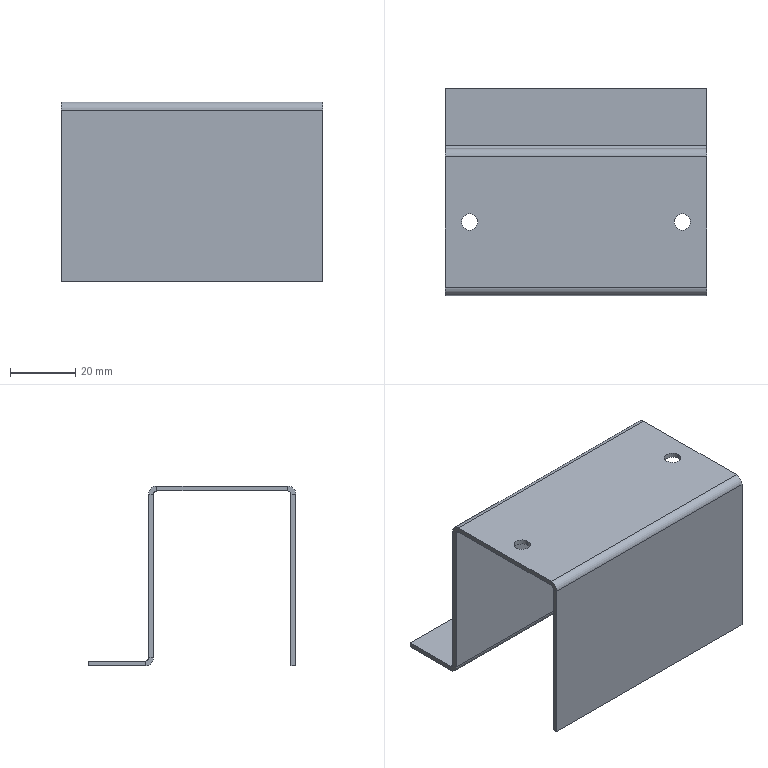Part | SolidWorks | features BaseBody 1 | 1 solid | 34 faces | box 80 x 63.5 x 55 mm | volume 20131 mm3 | plane 24 | cylinder 10 | commonest cylinder face diameters 5 x7 2 x3
STEP:
#1=CARTESIAN_POINT('',(-35.,0.,-1.5));
#2=VERTEX_POINT('',#1);
#3=CARTESIAN_POINT('',(-35.,0.,0.));
#4=VERTEX_POINT('',#3);
#5=CARTESIAN_POINT('',(-35.,0.,-1.5));
#6=DIRECTION('',(0.,0.,1.));
#7=VECTOR('',#6,1000.);
#8=LINE('',#5,#7);
#9=EDGE_CURVE('',#2,#4,#8,.T.);
#10=ORIENTED_EDGE('',*,*,#9,.F.);
#11=CARTESIAN_POINT('',(-30.,0.,-1.5));
#12=VERTEX_POINT('',#11);
#13=CARTESIAN_POINT('',(-32.5,0.,-1.5));
#14=DIRECTION('',(0.,0.,1.));
#15=DIRECTION('',(1.,0.,0.));
#16=AXIS2_PLACEMENT_3D('',#13,#14,#15);
#17=CIRCLE('',#16,2.5);
#18=EDGE_CURVE('',#12,#2,#17,.T.);
#19=ORIENTED_EDGE('',*,*,#18,.F.);
#20=CARTESIAN_POINT('',(-30.,0.,0.));
#21=VERTEX_POINT('',#20);
#22=CARTESIAN_POINT('',(-30.,0.,-1.5));
#23=DIRECTION('',(0.,0.,1.));
#24=VECTOR('',#23,1000.);
#25=LINE('',#22,#24);
#26=EDGE_CURVE('',#12,#21,#25,.T.);
#27=ORIENTED_EDGE('',*,*,#26,.T.);
#28=CARTESIAN_POINT('',(-32.5,0.,0.));
#29=DIRECTION('',(0.,0.,1.));
#30=DIRECTION('',(1.,0.,0.));
#31=AXIS2_PLACEMENT_3D('',#28,#29,#30);
#32=CIRCLE('',#31,2.5);
#33=EDGE_CURVE('',#21,#4,#32,.T.);
#34=ORIENTED_EDGE('',*,*,#33,.T.);
#35=EDGE_LOOP('',(#10,#19,#27,#34));
#36=FACE_OUTER_BOUND('',#35,.T.);
#37=CARTESIAN_POINT('',(-32.5,0.,-1.5));
#38=DIRECTION('',(0.,0.,1.));
#39=DIRECTION('',(1.,0.,0.));
#40=AXIS2_PLACEMENT_3D('',#37,#38,#39);
#41=CYLINDRICAL_SURFACE('',#40,2.5);
#42=ADVANCED_FACE('',(#36),#41,.F.);
#43=CARTESIAN_POINT('',(30.,0.,-1.5));
#44=VERTEX_POINT('',#43);
#45=CARTESIAN_POINT('',(30.,0.,0.));
#46=VERTEX_POINT('',#45);
#47=CARTESIAN_POINT('',(30.,0.,-1.5));
#48=DIRECTION('',(0.,0.,1.));
#49=VECTOR('',#48,1000.);
#50=LINE('',#47,#49);
#51=EDGE_CURVE('',#44,#46,#50,.T.);
#52=ORIENTED_EDGE('',*,*,#51,.F.);
#53=CARTESIAN_POINT('',(35.,0.,-1.5));
#54=VERTEX_POINT('',#53);
#55=CARTESIAN_POINT('',(32.5,0.,-1.5));
#56=DIRECTION('',(0.,0.,1.));
#57=DIRECTION('',(-1.,0.,0.));
#58=AXIS2_PLACEMENT_3D('',#55,#56,#57);
#59=CIRCLE('',#58,2.5);
#60=EDGE_CURVE('',#54,#44,#59,.T.);
#61=ORIENTED_EDGE('',*,*,#60,.F.);
#62=CARTESIAN_POINT('',(35.,0.,0.));
#63=VERTEX_POINT('',#62);
#64=CARTESIAN_POINT('',(35.,0.,-1.5));
#65=DIRECTION('',(0.,0.,1.));
#66=VECTOR('',#65,1000.);
#67=LINE('',#64,#66);
#68=EDGE_CURVE('',#54,#63,#67,.T.);
#69=ORIENTED_EDGE('',*,*,#68,.T.);
#70=CARTESIAN_POINT('',(32.5,0.,0.));
#71=DIRECTION('',(0.,0.,1.));
#72=DIRECTION('',(-1.,0.,0.));
#73=AXIS2_PLACEMENT_3D('',#70,#71,#72);
#74=CIRCLE('',#73,2.5);
#75=EDGE_CURVE('',#63,#46,#74,.T.);
#76=ORIENTED_EDGE('',*,*,#75,.T.);
#77=EDGE_LOOP('',(#52,#61,#69,#76));
#78=FACE_OUTER_BOUND('',#77,.T.);
#79=CARTESIAN_POINT('',(32.5,0.,-1.5));
#80=DIRECTION('',(0.,0.,1.));
#81=DIRECTION('',(1.,0.,0.));
#82=AXIS2_PLACEMENT_3D('',#79,#80,#81);
#83=CYLINDRICAL_SURFACE('',#82,2.5);
#84=ADVANCED_FACE('',(#78),#83,.F.);
#85=CARTESIAN_POINT('',(-40.,41.,-53.5));
#86=VERTEX_POINT('',#85);
#87=CARTESIAN_POINT('',(40.,41.,-53.5));
#88=VERTEX_POINT('',#87);
#89=CARTESIAN_POINT('',(40.,41.,-53.5));
#90=DIRECTION('',(1.,0.,0.));
#91=VECTOR('',#90,1000.);
#92=LINE('',#89,#91);
#93=EDGE_CURVE('',#86,#88,#92,.T.);
#94=ORIENTED_EDGE('',*,*,#93,.T.);
#95=CARTESIAN_POINT('',(40.,41.,-55.));
#96=VERTEX_POINT('',#95);
#97=CARTESIAN_POINT('',(40.,41.,-55.));
#98=DIRECTION('',(0.,0.,1.));
#99=VECTOR('',#98,1000.);
#100=LINE('',#97,#99);
#101=EDGE_CURVE('',#96,#88,#100,.T.);
#102=ORIENTED_EDGE('',*,*,#101,.F.);
#103=CARTESIAN_POINT('',(-40.,41.,-55.));
#104=VERTEX_POINT('',#103);
#105=CARTESIAN_POINT('',(0.,41.,-55.));
#106=DIRECTION('',(1.,0.,0.));
#107=VECTOR('',#106,1000.);
#108=LINE('',#105,#107);
#109=EDGE_CURVE('',#104,#96,#108,.T.);
#110=ORIENTED_EDGE('',*,*,#109,.F.);
#111=CARTESIAN_POINT('',(-40.,41.,-55.));
#112=DIRECTION('',(0.,0.,1.));
#113=VECTOR('',#112,1000.);
#114=LINE('',#111,#113);
#115=EDGE_CURVE('',#104,#86,#114,.T.);
#116=ORIENTED_EDGE('',*,*,#115,.T.);
#117=EDGE_LOOP('',(#94,#102,#110,#116));
#118=FACE_OUTER_BOUND('',#117,.T.);
#119=CARTESIAN_POINT('',(40.,41.,-55.));
#120=DIRECTION('',(0.,-1.,0.));
#121=DIRECTION('',(0.,0.,-1.));
#122=AXIS2_PLACEMENT_3D('',#119,#120,#121);
#123=PLANE('',#122);
#124=ADVANCED_FACE('',(#118),#123,.F.);
#125=CARTESIAN_POINT('',(-40.,23.5,-53.5));
#126=VERTEX_POINT('',#125);
#127=CARTESIAN_POINT('',(-40.,41.,-53.5));
#128=DIRECTION('',(0.,1.,0.));
#129=VECTOR('',#128,1000.);
#130=LINE('',#127,#129);
#131=EDGE_CURVE('',#126,#86,#130,.T.);
#132=ORIENTED_EDGE('',*,*,#131,.F.);
#133=CARTESIAN_POINT('',(40.,23.5,-53.5));
#134=VERTEX_POINT('',#133);
#135=CARTESIAN_POINT('',(40.,23.5,-53.5));
#136=DIRECTION('',(-1.,0.,0.));
#137=VECTOR('',#136,1000.);
#138=LINE('',#135,#137);
#139=EDGE_CURVE('',#134,#126,#138,.T.);
#140=ORIENTED_EDGE('',*,*,#139,.F.);
#141=CARTESIAN_POINT('',(40.,22.5,-53.5));
#142=DIRECTION('',(0.,-1.,0.));
#143=VECTOR('',#142,1000.);
#144=LINE('',#141,#143);
#145=EDGE_CURVE('',#88,#134,#144,.T.);
#146=ORIENTED_EDGE('',*,*,#145,.F.);
#147=ORIENTED_EDGE('',*,*,#93,.F.);
#148=EDGE_LOOP('',(#132,#140,#146,#147));
#149=FACE_OUTER_BOUND('',#148,.T.);
#150=CARTESIAN_POINT('',(0.,0.,-53.5));
#151=DIRECTION('',(0.,0.,1.));
#152=DIRECTION('',(1.,0.,0.));
#153=AXIS2_PLACEMENT_3D('',#150,#151,#152);
#154=PLANE('',#153);
#155=ADVANCED_FACE('',(#149),#154,.T.);
#156=CARTESIAN_POINT('',(-40.,23.5,-55.));
#157=VERTEX_POINT('',#156);
#158=CARTESIAN_POINT('',(40.,23.5,-55.));
#159=VERTEX_POINT('',#158);
#160=CARTESIAN_POINT('',(40.,23.5,-55.));
#161=DIRECTION('',(1.,0.,0.));
#162=VECTOR('',#161,1000.);
#163=LINE('',#160,#162);
#164=EDGE_CURVE('',#157,#159,#163,.T.);
#165=ORIENTED_EDGE('',*,*,#164,.F.);
#166=CARTESIAN_POINT('',(-40.,0.,-55.));
#167=DIRECTION('',(0.,1.,0.));
#168=VECTOR('',#167,1000.);
#169=LINE('',#166,#168);
#170=EDGE_CURVE('',#157,#104,#169,.T.);
#171=ORIENTED_EDGE('',*,*,#170,.T.);
#172=ORIENTED_EDGE('',*,*,#109,.T.);
#173=CARTESIAN_POINT('',(40.,0.,-55.));
#174=DIRECTION('',(0.,-1.,0.));
#175=VECTOR('',#174,1000.);
#176=LINE('',#173,#175);
#177=EDGE_CURVE('',#96,#159,#176,.T.);
#178=ORIENTED_EDGE('',*,*,#177,.T.);
#179=EDGE_LOOP('',(#165,#171,#172,#178));
#180=FACE_OUTER_BOUND('',#179,.T.);
#181=CARTESIAN_POINT('',(0.,0.,-55.));
#182=DIRECTION('',(0.,0.,1.));
#183=DIRECTION('',(1.,0.,0.));
#184=AXIS2_PLACEMENT_3D('',#181,#182,#183);
#185=PLANE('',#184);
#186=ADVANCED_FACE('',(#180),#185,.F.);
#187=CARTESIAN_POINT('',(-40.,23.5,-53.5));
#188=DIRECTION('',(0.,0.,-1.));
#189=VECTOR('',#188,1000.);
#190=LINE('',#187,#189);
#191=EDGE_CURVE('',#126,#157,#190,.T.);
#192=ORIENTED_EDGE('',*,*,#191,.F.);
#193=ORIENTED_EDGE('',*,*,#131,.T.);
#194=ORIENTED_EDGE('',*,*,#115,.F.);
#195=ORIENTED_EDGE('',*,*,#170,.F.);
#196=EDGE_LOOP('',(#192,#193,#194,#195));
#197=FACE_OUTER_BOUND('',#196,.T.);
#198=CARTESIAN_POINT('',(-40.,41.,-55.));
#199=DIRECTION('',(1.,0.,0.));
#200=DIRECTION('',(0.,1.,0.));
#201=AXIS2_PLACEMENT_3D('',#198,#199,#200);
#202=PLANE('',#201);
#203=ADVANCED_FACE('',(#197),#202,.F.);
#204=CARTESIAN_POINT('',(40.,23.5,-55.));
#205=DIRECTION('',(0.,0.,-1.));
#206=VECTOR('',#205,1000.);
#207=LINE('',#204,#206);
#208=EDGE_CURVE('',#134,#159,#207,.T.);
#209=ORIENTED_EDGE('',*,*,#208,.T.);
#210=ORIENTED_EDGE('',*,*,#177,.F.);
#211=ORIENTED_EDGE('',*,*,#101,.T.);
#212=ORIENTED_EDGE('',*,*,#145,.T.);
#213=EDGE_LOOP('',(#209,#210,#211,#212));
#214=FACE_OUTER_BOUND('',#213,.T.);
#215=CARTESIAN_POINT('',(40.,22.5,-55.));
#216=DIRECTION('',(-1.,0.,0.));
#217=DIRECTION('',(0.,0.,1.));
#218=AXIS2_PLACEMENT_3D('',#215,#216,#217);
#219=PLANE('',#218);
#220=ADVANCED_FACE('',(#214),#219,.F.);
#221=CARTESIAN_POINT('',(-40.,22.5,-52.5));
#222=VERTEX_POINT('',#221);
#223=CARTESIAN_POINT('',(40.,22.5,-52.5));
#224=VERTEX_POINT('',#223);
#225=CARTESIAN_POINT('',(-40.,22.5,-52.5));
#226=DIRECTION('',(1.,0.,0.));
#227=VECTOR('',#226,1000.);
#228=LINE('',#225,#227);
#229=EDGE_CURVE('',#222,#224,#228,.T.);
#230=ORIENTED_EDGE('',*,*,#229,.T.);
#231=CARTESIAN_POINT('',(40.,23.5,-52.5));
#232=DIRECTION('',(1.,0.,0.));
#233=DIRECTION('',(0.,0.,1.));
#234=AXIS2_PLACEMENT_3D('',#231,#232,#233);
#235=CIRCLE('',#234,1.);
#236=EDGE_CURVE('',#224,#134,#235,.T.);
#237=ORIENTED_EDGE('',*,*,#236,.T.);
#238=ORIENTED_EDGE('',*,*,#139,.T.);
#239=CARTESIAN_POINT('',(-40.,23.5,-52.5));
#240=DIRECTION('',(-1.,0.,0.));
#241=DIRECTION('',(0.,0.,1.));
#242=AXIS2_PLACEMENT_3D('',#239,#240,#241);
#243=CIRCLE('',#242,1.);
#244=EDGE_CURVE('',#126,#222,#243,.T.);
#245=ORIENTED_EDGE('',*,*,#244,.T.);
#246=EDGE_LOOP('',(#230,#237,#238,#245));
#247=FACE_OUTER_BOUND('',#246,.T.);
#248=CARTESIAN_POINT('',(-40.,23.5,-52.5));
#249=DIRECTION('',(-1.,0.,0.));
#250=DIRECTION('',(0.,0.,-1.));
#251=AXIS2_PLACEMENT_3D('',#248,#249,#250);
#252=CYLINDRICAL_SURFACE('',#251,1.);
#253=ADVANCED_FACE('',(#247),#252,.F.);
#254=CARTESIAN_POINT('',(-40.,21.,-52.5));
#255=VERTEX_POINT('',#254);
#256=CARTESIAN_POINT('',(40.,21.,-52.5));
#257=VERTEX_POINT('',#256);
#258=CARTESIAN_POINT('',(-40.,21.,-52.5));
#259=DIRECTION('',(1.,0.,0.));
#260=VECTOR('',#259,1000.);
#261=LINE('',#258,#260);
#262=EDGE_CURVE('',#255,#257,#261,.T.);
#263=ORIENTED_EDGE('',*,*,#262,.F.);
#264=CARTESIAN_POINT('',(-40.,23.5,-52.5));
#265=DIRECTION('',(-1.,0.,0.));
#266=DIRECTION('',(0.,0.,1.));
#267=AXIS2_PLACEMENT_3D('',#264,#265,#266);
#268=CIRCLE('',#267,2.5);
#269=EDGE_CURVE('',#157,#255,#268,.T.);
#270=ORIENTED_EDGE('',*,*,#269,.F.);
#271=ORIENTED_EDGE('',*,*,#164,.T.);
#272=CARTESIAN_POINT('',(40.,23.5,-52.5));
#273=DIRECTION('',(1.,0.,0.));
#274=DIRECTION('',(0.,0.,1.));
#275=AXIS2_PLACEMENT_3D('',#272,#273,#274);
#276=CIRCLE('',#275,2.5);
#277=EDGE_CURVE('',#257,#159,#276,.T.);
#278=ORIENTED_EDGE('',*,*,#277,.F.);
#279=EDGE_LOOP('',(#263,#270,#271,#278));
#280=FACE_OUTER_BOUND('',#279,.T.);
#281=CARTESIAN_POINT('',(-40.,23.5,-52.5));
#282=DIRECTION('',(-1.,0.,0.));
#283=DIRECTION('',(0.,0.,-1.));
#284=AXIS2_PLACEMENT_3D('',#281,#282,#283);
#285=CYLINDRICAL_SURFACE('',#284,2.5);
#286=ADVANCED_FACE('',(#280),#285,.T.);
#287=ORIENTED_EDGE('',*,*,#244,.F.);
#288=ORIENTED_EDGE('',*,*,#191,.T.);
#289=ORIENTED_EDGE('',*,*,#269,.T.);
#290=CARTESIAN_POINT('',(-40.,22.5,-52.5));
#291=DIRECTION('',(0.,-1.,0.));
#292=VECTOR('',#291,1000.);
#293=LINE('',#290,#292);
#294=EDGE_CURVE('',#222,#255,#293,.T.);
#295=ORIENTED_EDGE('',*,*,#294,.F.);
#296=EDGE_LOOP('',(#287,#288,#289,#295));
#297=FACE_OUTER_BOUND('',#296,.T.);
#298=CARTESIAN_POINT('',(-40.,23.5,-52.5));
#299=DIRECTION('',(1.,0.,0.));
#300=DIRECTION('',(0.,1.,0.));
#301=AXIS2_PLACEMENT_3D('',#298,#299,#300);
#302=PLANE('',#301);
#303=ADVANCED_FACE('',(#297),#302,.F.);
#304=ORIENTED_EDGE('',*,*,#208,.F.);
#305=ORIENTED_EDGE('',*,*,#236,.F.);
#306=CARTESIAN_POINT('',(40.,22.5,-52.5));
#307=DIRECTION('',(0.,-1.,0.));
#308=VECTOR('',#307,1000.);
#309=LINE('',#306,#308);
#310=EDGE_CURVE('',#224,#257,#309,.T.);
#311=ORIENTED_EDGE('',*,*,#310,.T.);
#312=ORIENTED_EDGE('',*,*,#277,.T.);
#313=EDGE_LOOP('',(#304,#305,#311,#312));
#314=FACE_OUTER_BOUND('',#313,.T.);
#315=CARTESIAN_POINT('',(40.,23.5,-52.5));
#316=DIRECTION('',(1.,0.,0.));
#317=DIRECTION('',(0.,1.,0.));
#318=AXIS2_PLACEMENT_3D('',#315,#316,#317);
#319=PLANE('',#318);
#320=ADVANCED_FACE('',(#314),#319,.T.);
#321=CARTESIAN_POINT('',(40.,20.,-1.5));
#322=VERTEX_POINT('',#321);
#323=CARTESIAN_POINT('',(-40.,20.,-1.5));
#324=VERTEX_POINT('',#323);
#325=CARTESIAN_POINT('',(40.,20.,-1.5));
#326=DIRECTION('',(-1.,0.,0.));
#327=VECTOR('',#326,1000.);
#328=LINE('',#325,#327);
#329=EDGE_CURVE('',#322,#324,#328,.T.);
#330=ORIENTED_EDGE('',*,*,#329,.T.);
#331=CARTESIAN_POINT('',(-40.,21.,-2.5));
#332=VERTEX_POINT('',#331);
#333=CARTESIAN_POINT('',(-40.,20.,-2.5));
#334=DIRECTION('',(-1.,0.,0.));
#335=DIRECTION('',(0.,0.,-1.));
#336=AXIS2_PLACEMENT_3D('',#333,#334,#335);
#337=CIRCLE('',#336,1.);
#338=EDGE_CURVE('',#324,#332,#337,.T.);
#339=ORIENTED_EDGE('',*,*,#338,.T.);
#340=CARTESIAN_POINT('',(40.,21.,-2.5));
#341=VERTEX_POINT('',#340);
#342=CARTESIAN_POINT('',(-40.,21.,-2.5));
#343=DIRECTION('',(1.,0.,0.));
#344=VECTOR('',#343,1000.);
#345=LINE('',#342,#344);
#346=EDGE_CURVE('',#332,#341,#345,.T.);
#347=ORIENTED_EDGE('',*,*,#346,.T.);
#348=CARTESIAN_POINT('',(40.,20.,-2.5));
#349=DIRECTION('',(1.,0.,0.));
#350=DIRECTION('',(0.,0.,-1.));
#351=AXIS2_PLACEMENT_3D('',#348,#349,#350);
#352=CIRCLE('',#351,1.);
#353=EDGE_CURVE('',#341,#322,#352,.T.);
#354=ORIENTED_EDGE('',*,*,#353,.T.);
#355=EDGE_LOOP('',(#330,#339,#347,#354));
#356=FACE_OUTER_BOUND('',#355,.T.);
#357=CARTESIAN_POINT('',(40.,20.,-2.5));
#358=DIRECTION('',(1.,0.,0.));
#359=DIRECTION('',(0.,1.,0.));
#360=AXIS2_PLACEMENT_3D('',#357,#358,#359);
#361=CYLINDRICAL_SURFACE('',#360,1.);
#362=ADVANCED_FACE('',(#356),#361,.F.);
#363=CARTESIAN_POINT('',(40.,20.,0.));
#364=VERTEX_POINT('',#363);
#365=CARTESIAN_POINT('',(-40.,20.,0.));
#366=VERTEX_POINT('',#365);
#367=CARTESIAN_POINT('',(40.,20.,0.));
#368=DIRECTION('',(-1.,0.,0.));
#369=VECTOR('',#368,1000.);
#370=LINE('',#367,#369);
#371=EDGE_CURVE('',#364,#366,#370,.T.);
#372=ORIENTED_EDGE('',*,*,#371,.F.);
#373=CARTESIAN_POINT('',(40.,22.5,-2.5));
#374=VERTEX_POINT('',#373);
#375=CARTESIAN_POINT('',(40.,20.,-2.5));
#376=DIRECTION('',(1.,0.,0.));
#377=DIRECTION('',(0.,0.,-1.));
#378=AXIS2_PLACEMENT_3D('',#375,#376,#377);
#379=CIRCLE('',#378,2.5);
#380=EDGE_CURVE('',#374,#364,#379,.T.);
#381=ORIENTED_EDGE('',*,*,#380,.F.);
#382=CARTESIAN_POINT('',(-40.,22.5,-2.5));
#383=VERTEX_POINT('',#382);
#384=CARTESIAN_POINT('',(-40.,22.5,-2.5));
#385=DIRECTION('',(-1.,0.,0.));
#386=VECTOR('',#385,1000.);
#387=LINE('',#384,#386);
#388=EDGE_CURVE('',#374,#383,#387,.T.);
#389=ORIENTED_EDGE('',*,*,#388,.T.);
#390=CARTESIAN_POINT('',(-40.,20.,-2.5));
#391=DIRECTION('',(-1.,0.,0.));
#392=DIRECTION('',(0.,0.,-1.));
#393=AXIS2_PLACEMENT_3D('',#390,#391,#392);
#394=CIRCLE('',#393,2.5);
#395=EDGE_CURVE('',#366,#383,#394,.T.);
#396=ORIENTED_EDGE('',*,*,#395,.F.);
#397=EDGE_LOOP('',(#372,#381,#389,#396));
#398=FACE_OUTER_BOUND('',#397,.T.);
#399=CARTESIAN_POINT('',(40.,20.,-2.5));
#400=DIRECTION('',(1.,0.,0.));
#401=DIRECTION('',(0.,1.,0.));
#402=AXIS2_PLACEMENT_3D('',#399,#400,#401);
#403=CYLINDRICAL_SURFACE('',#402,2.5);
#404=ADVANCED_FACE('',(#398),#403,.T.);
#405=ORIENTED_EDGE('',*,*,#353,.F.);
#406=CARTESIAN_POINT('',(40.,21.,-2.5));
#407=DIRECTION('',(0.,1.,0.));
#408=VECTOR('',#407,1000.);
#409=LINE('',#406,#408);
#410=EDGE_CURVE('',#341,#374,#409,.T.);
#411=ORIENTED_EDGE('',*,*,#410,.T.);
#412=ORIENTED_EDGE('',*,*,#380,.T.);
#413=CARTESIAN_POINT('',(40.,20.,-1.5));
#414=DIRECTION('',(0.,0.,1.));
#415=VECTOR('',#414,1000.);
#416=LINE('',#413,#415);
#417=EDGE_CURVE('',#322,#364,#416,.T.);
#418=ORIENTED_EDGE('',*,*,#417,.F.);
#419=EDGE_LOOP('',(#405,#411,#412,#418));
#420=FACE_OUTER_BOUND('',#419,.T.);
#421=CARTESIAN_POINT('',(40.,20.,-2.5));
#422=DIRECTION('',(-1.,0.,0.));
#423=DIRECTION('',(0.,0.,1.));
#424=AXIS2_PLACEMENT_3D('',#421,#422,#423);
#425=PLANE('',#424);
#426=ADVANCED_FACE('',(#420),#425,.F.);
#427=CARTESIAN_POINT('',(-40.,22.5,-2.5));
#428=DIRECTION('',(0.,1.,0.));
#429=VECTOR('',#428,1000.);
#430=LINE('',#427,#429);
#431=EDGE_CURVE('',#332,#383,#430,.T.);
#432=ORIENTED_EDGE('',*,*,#431,.F.);
#433=ORIENTED_EDGE('',*,*,#338,.F.);
#434=CARTESIAN_POINT('',(-40.,20.,-1.5));
#435=DIRECTION('',(0.,0.,1.));
#436=VECTOR('',#435,1000.);
#437=LINE('',#434,#436);
#438=EDGE_CURVE('',#324,#366,#437,.T.);
#439=ORIENTED_EDGE('',*,*,#438,.T.);
#440=ORIENTED_EDGE('',*,*,#395,.T.);
#441=EDGE_LOOP('',(#432,#433,#439,#440));
#442=FACE_OUTER_BOUND('',#441,.T.);
#443=CARTESIAN_POINT('',(-40.,20.,-2.5));
#444=DIRECTION('',(-1.,0.,0.));
#445=DIRECTION('',(0.,0.,1.));
#446=AXIS2_PLACEMENT_3D('',#443,#444,#445);
#447=PLANE('',#446);
#448=ADVANCED_FACE('',(#442),#447,.T.);
#449=CARTESIAN_POINT('',(-40.,-21.,-55.));
#450=VERTEX_POINT('',#449);
#451=CARTESIAN_POINT('',(40.,-21.,-55.));
#452=VERTEX_POINT('',#451);
#453=CARTESIAN_POINT('',(40.,-21.,-55.));
#454=DIRECTION('',(1.,0.,0.));
#455=VECTOR('',#454,1000.);
#456=LINE('',#453,#455);
#457=EDGE_CURVE('',#450,#452,#456,.T.);
#458=ORIENTED_EDGE('',*,*,#457,.T.);
#459=CARTESIAN_POINT('',(40.,-22.5,-55.));
#460=VERTEX_POINT('',#459);
#461=CARTESIAN_POINT('',(40.,-22.5,-55.));
#462=DIRECTION('',(0.,1.,0.));
#463=VECTOR('',#462,1000.);
#464=LINE('',#461,#463);
#465=EDGE_CURVE('',#460,#452,#464,.T.);
#466=ORIENTED_EDGE('',*,*,#465,.F.);
#467=CARTESIAN_POINT('',(-40.,-22.5,-55.));
#468=VERTEX_POINT('',#467);
#469=CARTESIAN_POINT('',(0.,-22.5,-55.));
#470=DIRECTION('',(1.,0.,0.));
#471=VECTOR('',#470,1000.);
#472=LINE('',#469,#471);
#473=EDGE_CURVE('',#468,#460,#472,.T.);
#474=ORIENTED_EDGE('',*,*,#473,.F.);
#475=CARTESIAN_POINT('',(-40.,-22.5,-55.));
#476=DIRECTION('',(0.,1.,0.));
#477=VECTOR('',#476,1000.);
#478=LINE('',#475,#477);
#479=EDGE_CURVE('',#468,#450,#478,.T.);
#480=ORIENTED_EDGE('',*,*,#479,.T.);
#481=EDGE_LOOP('',(#458,#466,#474,#480));
#482=FACE_OUTER_BOUND('',#481,.T.);
#483=CARTESIAN_POINT('',(40.,-22.5,-55.));
#484=DIRECTION('',(0.,0.,1.));
#485=DIRECTION('',(0.,-1.,0.));
#486=AXIS2_PLACEMENT_3D('',#483,#484,#485);
#487=PLANE('',#486);
#488=ADVANCED_FACE('',(#482),#487,.F.);
#489=CARTESIAN_POINT('',(-40.,-21.,-2.5));
#490=VERTEX_POINT('',#489);
#491=CARTESIAN_POINT('',(-40.,-21.,-55.));
#492=DIRECTION('',(0.,0.,-1.));
#493=VECTOR('',#492,1000.);
#494=LINE('',#491,#493);
#495=EDGE_CURVE('',#490,#450,#494,.T.);
#496=ORIENTED_EDGE('',*,*,#495,.F.);
#497=CARTESIAN_POINT('',(40.,-21.,-2.5));
#498=VERTEX_POINT('',#497);
#499=CARTESIAN_POINT('',(40.,-21.,-2.5));
#500=DIRECTION('',(-1.,0.,0.));
#501=VECTOR('',#500,1000.);
#502=LINE('',#499,#501);
#503=EDGE_CURVE('',#498,#490,#502,.T.);
#504=ORIENTED_EDGE('',*,*,#503,.F.);
#505=CARTESIAN_POINT('',(40.,-21.,-1.5));
#506=DIRECTION('',(0.,0.,1.));
#507=VECTOR('',#506,1000.);
#508=LINE('',#505,#507);
#509=EDGE_CURVE('',#452,#498,#508,.T.);
#510=ORIENTED_EDGE('',*,*,#509,.F.);
#511=ORIENTED_EDGE('',*,*,#457,.F.);
#512=EDGE_LOOP('',(#496,#504,#510,#511));
#513=FACE_OUTER_BOUND('',#512,.T.);
#514=CARTESIAN_POINT('',(0.,-21.,0.));
#515=DIRECTION('',(0.,1.,0.));
#516=DIRECTION('',(0.,0.,-1.));
#517=AXIS2_PLACEMENT_3D('',#514,#515,#516);
#518=PLANE('',#517);
#519=ADVANCED_FACE('',(#513),#518,.T.);
#520=CARTESIAN_POINT('',(-40.,-22.5,-2.5));
#521=VERTEX_POINT('',#520);
#522=CARTESIAN_POINT('',(40.,-22.5,-2.5));
#523=VERTEX_POINT('',#522);
#524=CARTESIAN_POINT('',(40.,-22.5,-2.5));
#525=DIRECTION('',(1.,0.,0.));
#526=VECTOR('',#525,1000.);
#527=LINE('',#524,#526);
#528=EDGE_CURVE('',#521,#523,#527,.T.);
#529=ORIENTED_EDGE('',*,*,#528,.F.);
#530=CARTESIAN_POINT('',(-40.,-22.5,0.));
#531=DIRECTION('',(0.,0.,-1.));
#532=VECTOR('',#531,1000.);
#533=LINE('',#530,#532);
#534=EDGE_CURVE('',#521,#468,#533,.T.);
#535=ORIENTED_EDGE('',*,*,#534,.T.);
#536=ORIENTED_EDGE('',*,*,#473,.T.);
#537=CARTESIAN_POINT('',(40.,-22.5,0.));
#538=DIRECTION('',(0.,0.,1.));
#539=VECTOR('',#538,1000.);
#540=LINE('',#537,#539);
#541=EDGE_CURVE('',#460,#523,#540,.T.);
#542=ORIENTED_EDGE('',*,*,#541,.T.);
#543=EDGE_LOOP('',(#529,#535,#536,#542));
#544=FACE_OUTER_BOUND('',#543,.T.);
#545=CARTESIAN_POINT('',(0.,-22.5,0.));
#546=DIRECTION('',(0.,1.,0.));
#547=DIRECTION('',(0.,0.,-1.));
#548=AXIS2_PLACEMENT_3D('',#545,#546,#547);
#549=PLANE('',#548);
#550=ADVANCED_FACE('',(#544),#549,.F.);
#551=CARTESIAN_POINT('',(40.,-22.5,-2.5));
#552=DIRECTION('',(0.,-1.,0.));
#553=VECTOR('',#552,1000.);
#554=LINE('',#551,#553);
#555=EDGE_CURVE('',#498,#523,#554,.T.);
#556=ORIENTED_EDGE('',*,*,#555,.T.);
#557=ORIENTED_EDGE('',*,*,#541,.F.);
#558=ORIENTED_EDGE('',*,*,#465,.T.);
#559=ORIENTED_EDGE('',*,*,#509,.T.);
#560=EDGE_LOOP('',(#556,#557,#558,#559));
#561=FACE_OUTER_BOUND('',#560,.T.);
#562=CARTESIAN_POINT('',(40.,-22.5,-1.5));
#563=DIRECTION('',(-1.,0.,0.));
#564=DIRECTION('',(0.,1.,0.));
#565=AXIS2_PLACEMENT_3D('',#562,#563,#564);
#566=PLANE('',#565);
#567=ADVANCED_FACE('',(#561),#566,.F.);
#568=CARTESIAN_POINT('',(-40.,-21.,-2.5));
#569=DIRECTION('',(0.,-1.,0.));
#570=VECTOR('',#569,1000.);
#571=LINE('',#568,#570);
#572=EDGE_CURVE('',#490,#521,#571,.T.);
#573=ORIENTED_EDGE('',*,*,#572,.F.);
#574=ORIENTED_EDGE('',*,*,#495,.T.);
#575=ORIENTED_EDGE('',*,*,#479,.F.);
#576=ORIENTED_EDGE('',*,*,#534,.F.);
#577=EDGE_LOOP('',(#573,#574,#575,#576));
#578=FACE_OUTER_BOUND('',#577,.T.);
#579=CARTESIAN_POINT('',(-40.,-22.5,-55.));
#580=DIRECTION('',(1.,0.,0.));
#581=DIRECTION('',(0.,1.,0.));
#582=AXIS2_PLACEMENT_3D('',#579,#580,#581);
#583=PLANE('',#582);
#584=ADVANCED_FACE('',(#578),#583,.F.);
#585=CARTESIAN_POINT('',(-40.,-20.,-1.5));
#586=VERTEX_POINT('',#585);
#587=CARTESIAN_POINT('',(40.,-20.,-1.5));
#588=VERTEX_POINT('',#587);
#589=CARTESIAN_POINT('',(-40.,-20.,-1.5));
#590=DIRECTION('',(1.,0.,0.));
#591=VECTOR('',#590,1000.);
#592=LINE('',#589,#591);
#593=EDGE_CURVE('',#586,#588,#592,.T.);
#594=ORIENTED_EDGE('',*,*,#593,.T.);
#595=CARTESIAN_POINT('',(40.,-20.,-2.5));
#596=DIRECTION('',(1.,0.,0.));
#597=DIRECTION('',(0.,0.,1.));
#598=AXIS2_PLACEMENT_3D('',#595,#596,#597);
#599=CIRCLE('',#598,1.);
#600=EDGE_CURVE('',#588,#498,#599,.T.);
#601=ORIENTED_EDGE('',*,*,#600,.T.);
#602=ORIENTED_EDGE('',*,*,#503,.T.);
#603=CARTESIAN_POINT('',(-40.,-20.,-2.5));
#604=DIRECTION('',(-1.,0.,0.));
#605=DIRECTION('',(0.,0.,1.));
#606=AXIS2_PLACEMENT_3D('',#603,#604,#605);
#607=CIRCLE('',#606,1.);
#608=EDGE_CURVE('',#490,#586,#607,.T.);
#609=ORIENTED_EDGE('',*,*,#608,.T.);
#610=EDGE_LOOP('',(#594,#601,#602,#609));
#611=FACE_OUTER_BOUND('',#610,.T.);
#612=CARTESIAN_POINT('',(-40.,-20.,-2.5));
#613=DIRECTION('',(-1.,0.,0.));
#614=DIRECTION('',(0.,-1.,0.));
#615=AXIS2_PLACEMENT_3D('',#612,#613,#614);
#616=CYLINDRICAL_SURFACE('',#615,1.);
#617=ADVANCED_FACE('',(#611),#616,.F.);
#618=CARTESIAN_POINT('',(-40.,-20.,0.));
#619=VERTEX_POINT('',#618);
#620=CARTESIAN_POINT('',(40.,-20.,0.));
#621=VERTEX_POINT('',#620);
#622=CARTESIAN_POINT('',(-40.,-20.,0.));
#623=DIRECTION('',(1.,0.,0.));
#624=VECTOR('',#623,1000.);
#625=LINE('',#622,#624);
#626=EDGE_CURVE('',#619,#621,#625,.T.);
#627=ORIENTED_EDGE('',*,*,#626,.F.);
#628=CARTESIAN_POINT('',(-40.,-20.,-2.5));
#629=DIRECTION('',(-1.,0.,0.));
#630=DIRECTION('',(0.,0.,1.));
#631=AXIS2_PLACEMENT_3D('',#628,#629,#630);
#632=CIRCLE('',#631,2.5);
#633=EDGE_CURVE('',#521,#619,#632,.T.);
#634=ORIENTED_EDGE('',*,*,#633,.F.);
#635=ORIENTED_EDGE('',*,*,#528,.T.);
#636=CARTESIAN_POINT('',(40.,-20.,-2.5));
#637=DIRECTION('',(1.,0.,0.));
#638=DIRECTION('',(0.,0.,1.));
#639=AXIS2_PLACEMENT_3D('',#636,#637,#638);
#640=CIRCLE('',#639,2.5);
#641=EDGE_CURVE('',#621,#523,#640,.T.);
#642=ORIENTED_EDGE('',*,*,#641,.F.);
#643=EDGE_LOOP('',(#627,#634,#635,#642));
#644=FACE_OUTER_BOUND('',#643,.T.);
#645=CARTESIAN_POINT('',(-40.,-20.,-2.5));
#646=DIRECTION('',(-1.,0.,0.));
#647=DIRECTION('',(0.,-1.,0.));
#648=AXIS2_PLACEMENT_3D('',#645,#646,#647);
#649=CYLINDRICAL_SURFACE('',#648,2.5);
#650=ADVANCED_FACE('',(#644),#649,.T.);
#651=ORIENTED_EDGE('',*,*,#608,.F.);
#652=ORIENTED_EDGE('',*,*,#572,.T.);
#653=ORIENTED_EDGE('',*,*,#633,.T.);
#654=CARTESIAN_POINT('',(-40.,-20.,-1.5));
#655=DIRECTION('',(0.,0.,1.));
#656=VECTOR('',#655,1000.);
#657=LINE('',#654,#656);
#658=EDGE_CURVE('',#586,#619,#657,.T.);
#659=ORIENTED_EDGE('',*,*,#658,.F.);
#660=EDGE_LOOP('',(#651,#652,#653,#659));
#661=FACE_OUTER_BOUND('',#660,.T.);
#662=CARTESIAN_POINT('',(-40.,-20.,-2.5));
#663=DIRECTION('',(1.,0.,0.));
#664=DIRECTION('',(0.,1.,0.));
#665=AXIS2_PLACEMENT_3D('',#662,#663,#664);
#666=PLANE('',#665);
#667=ADVANCED_FACE('',(#661),#666,.F.);
#668=ORIENTED_EDGE('',*,*,#555,.F.);
#669=ORIENTED_EDGE('',*,*,#600,.F.);
#670=CARTESIAN_POINT('',(40.,-20.,-1.5));
#671=DIRECTION('',(0.,0.,1.));
#672=VECTOR('',#671,1000.);
#673=LINE('',#670,#672);
#674=EDGE_CURVE('',#588,#621,#673,.T.);
#675=ORIENTED_EDGE('',*,*,#674,.T.);
#676=ORIENTED_EDGE('',*,*,#641,.T.);
#677=EDGE_LOOP('',(#668,#669,#675,#676));
#678=FACE_OUTER_BOUND('',#677,.T.);
#679=CARTESIAN_POINT('',(40.,-20.,-2.5));
#680=DIRECTION('',(1.,0.,0.));
#681=DIRECTION('',(0.,1.,0.));
#682=AXIS2_PLACEMENT_3D('',#679,#680,#681);
#683=PLANE('',#682);
#684=ADVANCED_FACE('',(#678),#683,.T.);
#685=ORIENTED_EDGE('',*,*,#438,.F.);
#686=CARTESIAN_POINT('',(-40.,22.5,-1.5));
#687=DIRECTION('',(0.,-1.,0.));
#688=VECTOR('',#687,1000.);
#689=LINE('',#686,#688);
#690=EDGE_CURVE('',#324,#586,#689,.T.);
#691=ORIENTED_EDGE('',*,*,#690,.T.);
#692=ORIENTED_EDGE('',*,*,#658,.T.);
#693=CARTESIAN_POINT('',(-40.,22.5,0.));
#694=DIRECTION('',(0.,-1.,0.));
#695=VECTOR('',#694,1000.);
#696=LINE('',#693,#695);
#697=EDGE_CURVE('',#366,#619,#696,.T.);
#698=ORIENTED_EDGE('',*,*,#697,.F.);
#699=EDGE_LOOP('',(#685,#691,#692,#698));
#700=FACE_OUTER_BOUND('',#699,.T.);
#701=CARTESIAN_POINT('',(-40.,22.5,-1.5));
#702=DIRECTION('',(-1.,0.,0.));
#703=DIRECTION('',(0.,0.,1.));
#704=AXIS2_PLACEMENT_3D('',#701,#702,#703);
#705=PLANE('',#704);
#706=ADVANCED_FACE('',(#700),#705,.T.);
#707=CARTESIAN_POINT('',(40.,22.5,-1.5));
#708=DIRECTION('',(0.,1.,0.));
#709=VECTOR('',#708,1000.);
#710=LINE('',#707,#709);
#711=EDGE_CURVE('',#588,#322,#710,.T.);
#712=ORIENTED_EDGE('',*,*,#711,.T.);
#713=ORIENTED_EDGE('',*,*,#417,.T.);
#714=CARTESIAN_POINT('',(40.,22.5,0.));
#715=DIRECTION('',(0.,1.,0.));
#716=VECTOR('',#715,1000.);
#717=LINE('',#714,#716);
#718=EDGE_CURVE('',#621,#364,#717,.T.);
#719=ORIENTED_EDGE('',*,*,#718,.F.);
#720=ORIENTED_EDGE('',*,*,#674,.F.);
#721=EDGE_LOOP('',(#712,#713,#719,#720));
#722=FACE_OUTER_BOUND('',#721,.T.);
#723=CARTESIAN_POINT('',(40.,22.5,-1.5));
#724=DIRECTION('',(1.,0.,0.));
#725=DIRECTION('',(0.,1.,0.));
#726=AXIS2_PLACEMENT_3D('',#723,#724,#725);
#727=PLANE('',#726);
#728=ADVANCED_FACE('',(#722),#727,.T.);
#729=ORIENTED_EDGE('',*,*,#75,.F.);
#730=CARTESIAN_POINT('',(32.5,0.,0.));
#731=DIRECTION('',(0.,0.,1.));
#732=DIRECTION('',(-1.,0.,0.));
#733=AXIS2_PLACEMENT_3D('',#730,#731,#732);
#734=CIRCLE('',#733,2.5);
#735=EDGE_CURVE('',#46,#63,#734,.T.);
#736=ORIENTED_EDGE('',*,*,#735,.F.);
#737=EDGE_LOOP('',(#729,#736));
#738=FACE_BOUND('',#737,.T.);
#739=ORIENTED_EDGE('',*,*,#33,.F.);
#740=CARTESIAN_POINT('',(-32.5,0.,0.));
#741=DIRECTION('',(0.,0.,1.));
#742=DIRECTION('',(1.,0.,0.));
#743=AXIS2_PLACEMENT_3D('',#740,#741,#742);
#744=CIRCLE('',#743,2.5);
#745=EDGE_CURVE('',#4,#21,#744,.T.);
#746=ORIENTED_EDGE('',*,*,#745,.F.);
#747=EDGE_LOOP('',(#739,#746));
#748=FACE_BOUND('',#747,.T.);
#749=ORIENTED_EDGE('',*,*,#371,.T.);
#750=ORIENTED_EDGE('',*,*,#697,.T.);
#751=ORIENTED_EDGE('',*,*,#626,.T.);
#752=ORIENTED_EDGE('',*,*,#718,.T.);
#753=EDGE_LOOP('',(#749,#750,#751,#752));
#754=FACE_OUTER_BOUND('',#753,.T.);
#755=CARTESIAN_POINT('',(0.,0.,0.));
#756=DIRECTION('',(0.,0.,-1.));
#757=DIRECTION('',(0.,-1.,0.));
#758=AXIS2_PLACEMENT_3D('',#755,#756,#757);
#759=PLANE('',#758);
#760=ADVANCED_FACE('',(#738,#748,#754),#759,.F.);
#761=ORIENTED_EDGE('',*,*,#60,.T.);
#762=CARTESIAN_POINT('',(32.5,0.,-1.5));
#763=DIRECTION('',(0.,0.,1.));
#764=DIRECTION('',(-1.,0.,0.));
#765=AXIS2_PLACEMENT_3D('',#762,#763,#764);
#766=CIRCLE('',#765,2.5);
#767=EDGE_CURVE('',#44,#54,#766,.T.);
#768=ORIENTED_EDGE('',*,*,#767,.T.);
#769=EDGE_LOOP('',(#761,#768));
#770=FACE_BOUND('',#769,.T.);
#771=ORIENTED_EDGE('',*,*,#18,.T.);
#772=CARTESIAN_POINT('',(-32.5,0.,-1.5));
#773=DIRECTION('',(0.,0.,1.));
#774=DIRECTION('',(1.,0.,0.));
#775=AXIS2_PLACEMENT_3D('',#772,#773,#774);
#776=CIRCLE('',#775,2.5);
#777=EDGE_CURVE('',#2,#12,#776,.T.);
#778=ORIENTED_EDGE('',*,*,#777,.T.);
#779=EDGE_LOOP('',(#771,#778));
#780=FACE_BOUND('',#779,.T.);
#781=ORIENTED_EDGE('',*,*,#690,.F.);
#782=ORIENTED_EDGE('',*,*,#329,.F.);
#783=ORIENTED_EDGE('',*,*,#711,.F.);
#784=ORIENTED_EDGE('',*,*,#593,.F.);
#785=EDGE_LOOP('',(#781,#782,#783,#784));
#786=FACE_OUTER_BOUND('',#785,.T.);
#787=CARTESIAN_POINT('',(0.,0.,-1.5));
#788=DIRECTION('',(0.,0.,-1.));
#789=DIRECTION('',(0.,-1.,0.));
#790=AXIS2_PLACEMENT_3D('',#787,#788,#789);
#791=PLANE('',#790);
#792=ADVANCED_FACE('',(#770,#780,#786),#791,.T.);
#793=CARTESIAN_POINT('',(-40.,21.,-1.5));
#794=DIRECTION('',(0.,0.,1.));
#795=VECTOR('',#794,1000.);
#796=LINE('',#793,#795);
#797=EDGE_CURVE('',#255,#332,#796,.T.);
#798=ORIENTED_EDGE('',*,*,#797,.F.);
#799=ORIENTED_EDGE('',*,*,#262,.T.);
#800=CARTESIAN_POINT('',(40.,21.,-55.));
#801=DIRECTION('',(0.,0.,-1.));
#802=VECTOR('',#801,1000.);
#803=LINE('',#800,#802);
#804=EDGE_CURVE('',#341,#257,#803,.T.);
#805=ORIENTED_EDGE('',*,*,#804,.F.);
#806=ORIENTED_EDGE('',*,*,#346,.F.);
#807=EDGE_LOOP('',(#798,#799,#805,#806));
#808=FACE_OUTER_BOUND('',#807,.T.);
#809=CARTESIAN_POINT('',(0.,21.,0.));
#810=DIRECTION('',(0.,-1.,0.));
#811=DIRECTION('',(0.,0.,-1.));
#812=AXIS2_PLACEMENT_3D('',#809,#810,#811);
#813=PLANE('',#812);
#814=ADVANCED_FACE('',(#808),#813,.T.);
#815=ORIENTED_EDGE('',*,*,#229,.F.);
#816=CARTESIAN_POINT('',(-40.,22.5,0.));
#817=DIRECTION('',(0.,0.,1.));
#818=VECTOR('',#817,1000.);
#819=LINE('',#816,#818);
#820=EDGE_CURVE('',#222,#383,#819,.T.);
#821=ORIENTED_EDGE('',*,*,#820,.T.);
#822=ORIENTED_EDGE('',*,*,#388,.F.);
#823=CARTESIAN_POINT('',(40.,22.5,0.));
#824=DIRECTION('',(0.,0.,-1.));
#825=VECTOR('',#824,1000.);
#826=LINE('',#823,#825);
#827=EDGE_CURVE('',#374,#224,#826,.T.);
#828=ORIENTED_EDGE('',*,*,#827,.T.);
#829=EDGE_LOOP('',(#815,#821,#822,#828));
#830=FACE_OUTER_BOUND('',#829,.T.);
#831=CARTESIAN_POINT('',(0.,22.5,0.));
#832=DIRECTION('',(0.,-1.,0.));
#833=DIRECTION('',(0.,0.,-1.));
#834=AXIS2_PLACEMENT_3D('',#831,#832,#833);
#835=PLANE('',#834);
#836=ADVANCED_FACE('',(#830),#835,.F.);
#837=ORIENTED_EDGE('',*,*,#294,.T.);
#838=ORIENTED_EDGE('',*,*,#797,.T.);
#839=ORIENTED_EDGE('',*,*,#431,.T.);
#840=ORIENTED_EDGE('',*,*,#820,.F.);
#841=EDGE_LOOP('',(#837,#838,#839,#840));
#842=FACE_OUTER_BOUND('',#841,.T.);
#843=CARTESIAN_POINT('',(-40.,22.5,-1.5));
#844=DIRECTION('',(1.,0.,0.));
#845=DIRECTION('',(0.,0.,-1.));
#846=AXIS2_PLACEMENT_3D('',#843,#844,#845);
#847=PLANE('',#846);
#848=ADVANCED_FACE('',(#842),#847,.F.);
#849=ORIENTED_EDGE('',*,*,#310,.F.);
#850=ORIENTED_EDGE('',*,*,#827,.F.);
#851=ORIENTED_EDGE('',*,*,#410,.F.);
#852=ORIENTED_EDGE('',*,*,#804,.T.);
#853=EDGE_LOOP('',(#849,#850,#851,#852));
#854=FACE_OUTER_BOUND('',#853,.T.);
#855=CARTESIAN_POINT('',(40.,22.5,-55.));
#856=DIRECTION('',(-1.,0.,0.));
#857=DIRECTION('',(0.,1.,0.));
#858=AXIS2_PLACEMENT_3D('',#855,#856,#857);
#859=PLANE('',#858);
#860=ADVANCED_FACE('',(#854),#859,.F.);
#861=ORIENTED_EDGE('',*,*,#767,.F.);
#862=ORIENTED_EDGE('',*,*,#51,.T.);
#863=ORIENTED_EDGE('',*,*,#735,.T.);
#864=ORIENTED_EDGE('',*,*,#68,.F.);
#865=EDGE_LOOP('',(#861,#862,#863,#864));
#866=FACE_OUTER_BOUND('',#865,.T.);
#867=CARTESIAN_POINT('',(32.5,0.,-1.5));
#868=DIRECTION('',(0.,0.,1.));
#869=DIRECTION('',(1.,0.,0.));
#870=AXIS2_PLACEMENT_3D('',#867,#868,#869);
#871=CYLINDRICAL_SURFACE('',#870,2.5);
#872=ADVANCED_FACE('',(#866),#871,.F.);
#873=ORIENTED_EDGE('',*,*,#777,.F.);
#874=ORIENTED_EDGE('',*,*,#9,.T.);
#875=ORIENTED_EDGE('',*,*,#745,.T.);
#876=ORIENTED_EDGE('',*,*,#26,.F.);
#877=EDGE_LOOP('',(#873,#874,#875,#876));
#878=FACE_OUTER_BOUND('',#877,.T.);
#879=CARTESIAN_POINT('',(-32.5,0.,-1.5));
#880=DIRECTION('',(0.,0.,1.));
#881=DIRECTION('',(1.,0.,0.));
#882=AXIS2_PLACEMENT_3D('',#879,#880,#881);
#883=CYLINDRICAL_SURFACE('',#882,2.5);
#884=ADVANCED_FACE('',(#878),#883,.F.);
#885=CLOSED_SHELL('',(#42,#84,#124,#155,#186,#203,#220,#253,#286,#303,#320,#362,#404,#426,#448,#488,#519,#550,#567,#584,#617,#650,#667,#684,#706,#728,#760,#792,#814,#836,#848,#860,#872,#884));
#886=MANIFOLD_SOLID_BREP('',#885);
#887=CARTESIAN_POINT('',(0.,0.,0.));
#888=DIRECTION('',(0.,0.,1.));
#889=DIRECTION('',(1.,0.,0.));
#890=AXIS2_PLACEMENT_3D('',#887,#888,#889);
#891=(LENGTH_UNIT()NAMED_UNIT(*)SI_UNIT(.MILLI.,.METRE.));
#892=UNCERTAINTY_MEASURE_WITH_UNIT(LENGTH_MEASURE(0.00001),#891,'','');
#893=(NAMED_UNIT(*)PLANE_ANGLE_UNIT()SI_UNIT($,.RADIAN.));
#894=(NAMED_UNIT(*)SI_UNIT($,.STERADIAN.)SOLID_ANGLE_UNIT());
#895=(GEOMETRIC_REPRESENTATION_CONTEXT(3)GLOBAL_UNCERTAINTY_ASSIGNED_CONTEXT((#892))GLOBAL_UNIT_ASSIGNED_CONTEXT((#891,#893,#894))REPRESENTATION_CONTEXT('',''));
#896=ADVANCED_BREP_SHAPE_REPRESENTATION('',(#886,#890),#895);